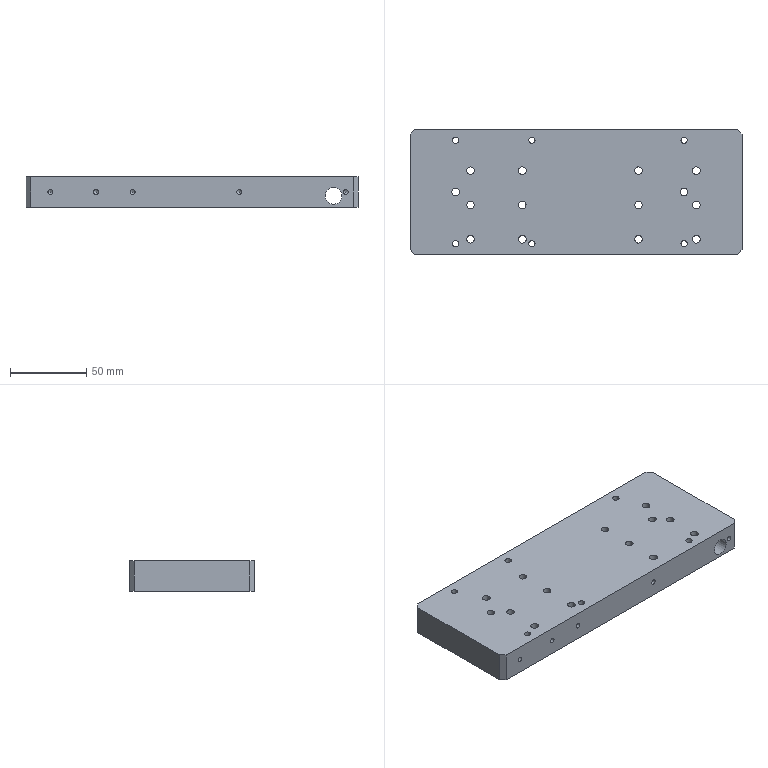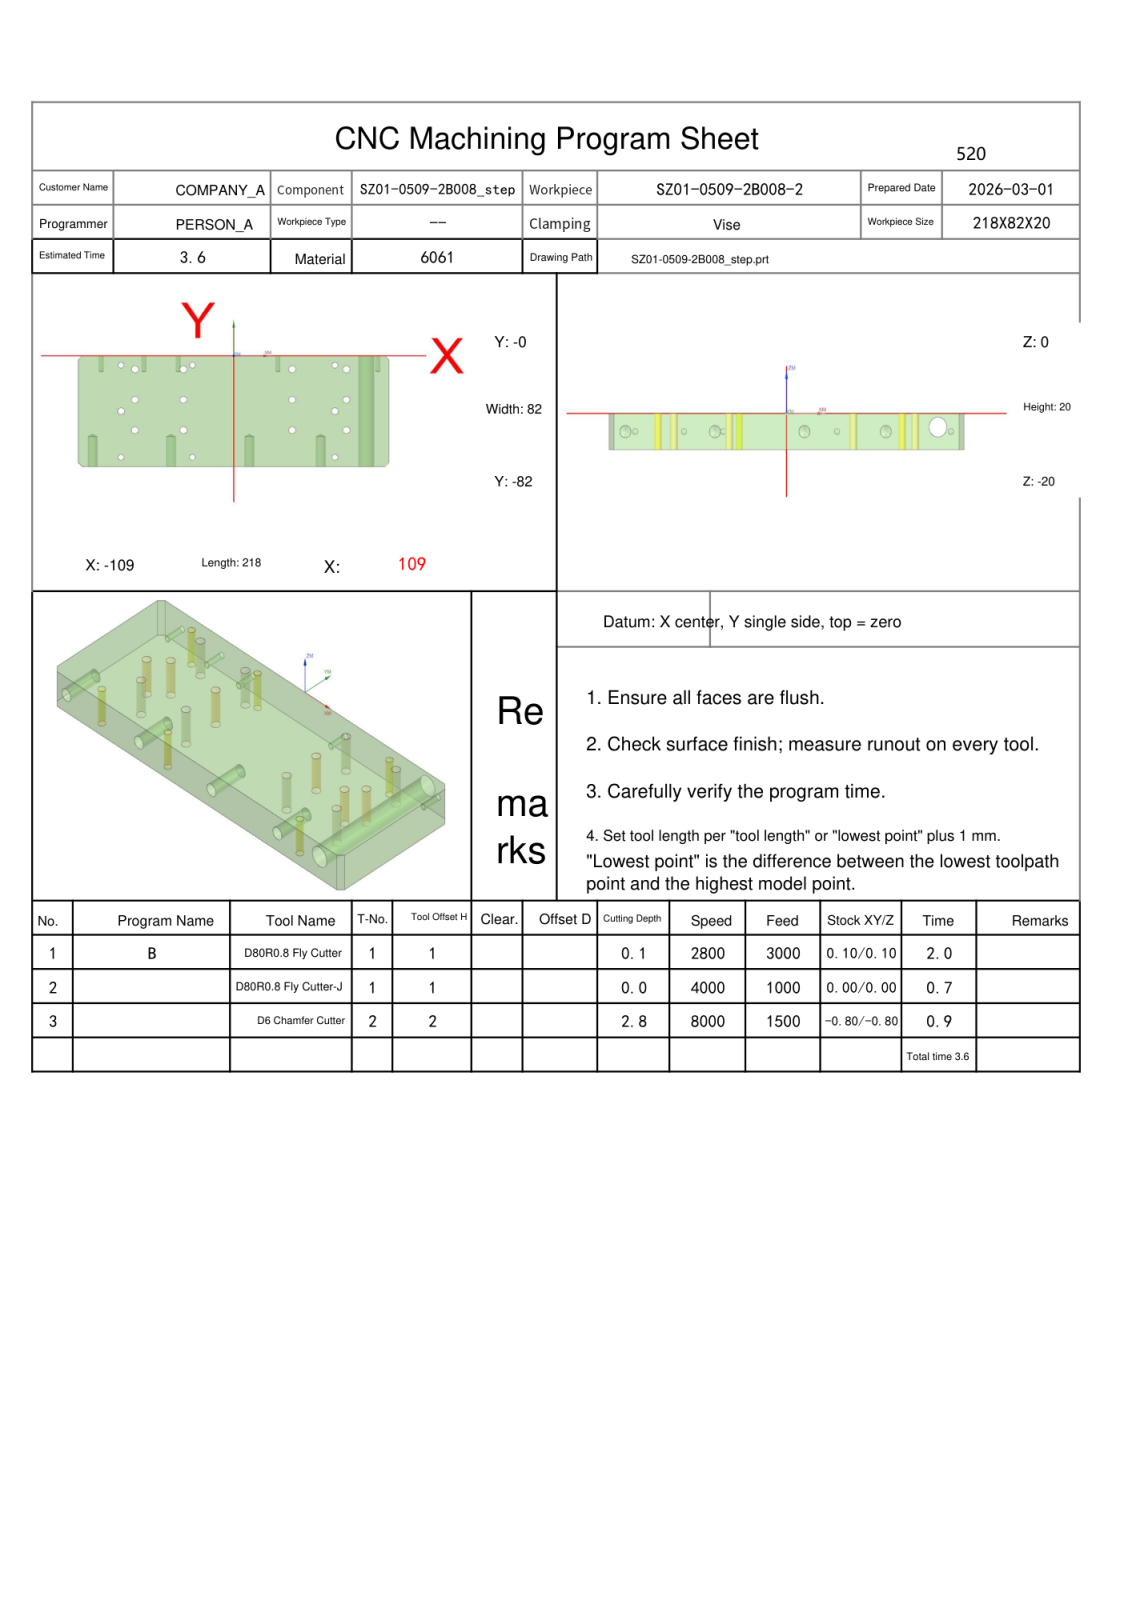NC program | NX | posted by the shop | part box 218 x 82 x 20 mm
Whole program:
%
O0001
(Machine time: 4.11 MIN)
(===Total Tool:2===)
(T1=D80R0.8 Fly Cutter D=80.  R=0.8  D-  H01 Z=0.    )
(T2=D6 Chamfer Cutter   D=6.   R=0.   D-  H02 Z=-2.8  )
G80 G90 G17 G49 G40
G91 G28 Z0
M01
N1 T01 M06
(D80R0.8 Fly Cutter  D=80. R=0.8 H=01 ce=0.10 di=0.10)
G00 G90 G54 X161.097 Y-58.097 M03 S2800
G43 H01 Z50.
M08
Z6.011
G01 Z4.011 F3000.
X149.097
X-141.897
G02 X-149.097 Y-50.897 I0.0 J7.2
G01 Y-39.263
G02 X-141.097 Y-31.263 I8. J0.0
G01 X149.097
X161.097
Z6.011
G00 Y-58.097
Z5.522
G01 Z3.522
X149.097
X-141.897
G02 X-149.097 Y-50.897 I0.0 J7.2
G01 Y-39.263
G02 X-141.097 Y-31.263 I8. J0.0
G01 X149.097
X161.097
Z5.522
G00 Y-58.097
Z5.033
G01 Z3.033
X149.097
X-141.897
G02 X-149.097 Y-50.897 I0.0 J7.2
G01 Y-39.263
G02 X-141.097 Y-31.263 I8. J0.0
G01 X149.097
X161.097
Z5.033
G00 Y-58.097
Z4.544
G01 Z2.544
X149.097
X-141.897
G02 X-149.097 Y-50.897 I0.0 J7.2
G01 Y-39.263
G02 X-141.097 Y-31.263 I8. J0.0
G01 X149.097
X161.097
Z4.544
G00 Y-58.097
Z4.056
G01 Z2.056
X149.097
X-141.897
G02 X-149.097 Y-50.897 I0.0 J7.2
G01 Y-39.263
G02 X-141.097 Y-31.263 I8. J0.0
G01 X149.097
X161.097
Z4.056
G00 Y-58.097
Z3.567
G01 Z1.567
X149.097
X-141.897
G02 X-149.097 Y-50.897 I0.0 J7.2
G01 Y-39.263
G02 X-141.097 Y-31.263 I8. J0.0
G01 X149.097
X161.097
Z3.567
G00 Y-58.097
Z3.078
G01 Z1.078
X149.097
X-141.897
G02 X-149.097 Y-50.897 I0.0 J7.2
G01 Y-39.263
G02 X-141.097 Y-31.263 I8. J0.0
G01 X149.097
X161.097
Z3.078
G00 Y-58.097
Z2.589
G01 Z.589
X149.097
X-141.897
G02 X-149.097 Y-50.897 I0.0 J7.2
G01 Y-39.263
G02 X-141.097 Y-31.263 I8. J0.0
G01 X149.097
X161.097
Z2.589
G00 Y-58.097
Z2.1
G01 Z.1
X149.097
X-141.897
G02 X-149.097 Y-50.897 I0.0 J7.2
G01 Y-39.263
G02 X-141.097 Y-31.263 I8. J0.0
G01 X149.097
X161.097
Z2.1
G00 Z50.
G91 G28 Z0.0
M05
M09
G91 G28 Z0.0
M01
N2 T01 M06
(D80R0.8 Fly Cutter-J  D=80. R=0.8 H=01 ce=0.00 di=0.00)
G00 G90 G54 X160.999 Y-57.999 M03 S4000
G43 H01 Z50.
M08
Z2.
G01 Z0.0 F1000.
X148.999
X-141.799
G02 X-148.999 Y-50.799 I0.0 J7.2
G01 Y-39.361
G02 X-140.999 Y-31.361 I8. J0.0
G01 X148.999
X160.999
Z2.
G00 Z50.
G91 G28 Z0.0
M05
M09
G91 G28 Z0.0
M01
N3 T02 M06
(D6 Chamfer Cutter  D=6. R=0. H=02 ce=0.00 di=0.00)
G00 G90 G54 X-29. Y-75. M03 S8000
G43 H02 Z50.
M08
G98 G81 X-29. Y-75. Z-2.7 R3. F1000.
X-79.
Y-7.
X-29.
X71.
Y-75.
G80
G00 Z50.
G00 G90 X-79. Y-41. M03 S8000
Z50.
G98 G81 X-79. Y-41. Z-2.8 R3. F1000.
X-69.275 Y-32.5
X-35.275
X41.
X71. Y-41.
X79. Y-32.5
G80
G00 Z50.
G00 G90 X41.273 Y-55.91 M03 S8000
Z50.
Z-.9
G01 Z-1.4 F600.
X41.45 Y-56.5
G03 X42.95 Y-55. I0.0 J1.5
X41. Y-53.05 I-1.95 J0.0
X39.05 Y-55. I0.0 J-1.95
X41. Y-56.95 I1.95 J0.0
X42.95 Y-55. I0.0 J1.95
X41.45 Y-53.5 I-1.5 J0.0
G01 X41.273 Y-54.09
Z-.9
G00 Z50.
X79.273 Y-55.91
Z-.9
G01 Z-1.4
X79.45 Y-56.5
G03 X80.95 Y-55. I0.0 J1.5
X79. Y-53.05 I-1.95 J0.0
X77.05 Y-55. I0.0 J-1.95
X79. Y-56.95 I1.95 J0.0
X80.95 Y-55. I0.0 J1.95
X79.45 Y-53.5 I-1.5 J0.0
G01 X79.273 Y-54.09
Z-.9
G00 Z50.
Y-10.91
Z-.9
G01 Z-1.4
X79.45 Y-11.5
G03 X80.95 Y-10. I0.0 J1.5
X79. Y-8.05 I-1.95 J0.0
X77.05 Y-10. I0.0 J-1.95
X79. Y-11.95 I1.95 J0.0
X80.95 Y-10. I0.0 J1.95
X79.45 Y-8.5 I-1.5 J0.0
G01 X79.273 Y-9.09
Z-.9
G00 Z50.
X41.273 Y-10.91
Z-.9
G01 Z-1.4
X41.45 Y-11.5
G03 X42.95 Y-10. I0.0 J1.5
X41. Y-8.05 I-1.95 J0.0
X39.05 Y-10. I0.0 J-1.95
X41. Y-11.95 I1.95 J0.0
X42.95 Y-10. I0.0 J1.95
X41.45 Y-8.5 I-1.5 J0.0
G01 X41.273 Y-9.09
Z-.9
G00 Z50.
X-35.002 Y-10.91
Z-.9
G01 Z-1.4
X-34.825 Y-11.5
G03 X-33.325 Y-10. I0.0 J1.5
X-35.275 Y-8.05 I-1.95 J0.0
X-37.225 Y-10. I0.0 J-1.95
X-35.275 Y-11.95 I1.95 J0.0
X-33.325 Y-10. I0.0 J1.95
X-34.825 Y-8.5 I-1.5 J0.0
G01 X-35.002 Y-9.09
Z-.9
G00 Z50.
X-69.002 Y-10.91
Z-.9
G01 Z-1.4
X-68.825 Y-11.5
G03 X-67.325 Y-10. I0.0 J1.5
X-69.275 Y-8.05 I-1.95 J0.0
X-71.225 Y-10. I0.0 J-1.95
X-69.275 Y-11.95 I1.95 J0.0
X-67.325 Y-10. I0.0 J1.95
X-68.825 Y-8.5 I-1.5 J0.0
G01 X-69.002 Y-9.09
Z-.9
G00 Z50.
Y-55.91
Z-.9
G01 Z-1.4
X-68.825 Y-56.5
G03 X-67.325 Y-55. I0.0 J1.5
X-69.275 Y-53.05 I-1.95 J0.0
X-71.225 Y-55. I0.0 J-1.95
X-69.275 Y-56.95 I1.95 J0.0
X-67.325 Y-55. I0.0 J1.95
X-68.825 Y-53.5 I-1.5 J0.0
G01 X-69.002 Y-54.09
Z-.9
G00 Z50.
X-35.002 Y-55.91
Z-.9
G01 Z-1.4
X-34.825 Y-56.5
G03 X-33.325 Y-55. I0.0 J1.5
X-35.275 Y-53.05 I-1.95 J0.0
X-37.225 Y-55. I0.0 J-1.95
X-35.275 Y-56.95 I1.95 J0.0
X-33.325 Y-55. I0.0 J1.95
X-34.825 Y-53.5 I-1.5 J0.0
G01 X-35.002 Y-54.09
Z-.9
G00 Z50.
G00 G90 X-97.046 Y-82.7 M03 S7000
Z50.
Z2.5
G01 X-105.876 Z-.714 F1500.
X-105.953 Z-.742
X-106.16 Y-82.662 Z-.819
X-106.355 Y-82.581 Z-.895
X-106.528 Y-82.462 Z-.972
X-106.583 Y-82.407 Z-1.
X-109.407 Y-79.583
G02 X-109.7 Y-78.876 I.707 J.707
G01 Y-3.124
G02 X-109.407 Y-2.417 I1. J0.0
G01 X-106.583 Y.407
G02 X-105.876 Y.7 I.707 J-.707
G01 X105.876
G02 X106.583 Y.407 I0.0 J-1.
G01 X109.407 Y-2.417
G02 X109.7 Y-3.124 I-.707 J-.707
G01 Y-78.876
G02 X109.407 Y-79.583 I-1. J0.0
G01 X106.583 Y-82.407
G02 X105.876 Y-82.7 I-.707 J.707
G01 X-105.876
G02 X-106.583 Y-82.407 I0.0 J1.
G01 X-106.936 Y-82.054
Z1.5
G00 Z50.
M05
M09
G91 G28 Z0.0
G91 G28 Y0.0
M30
%